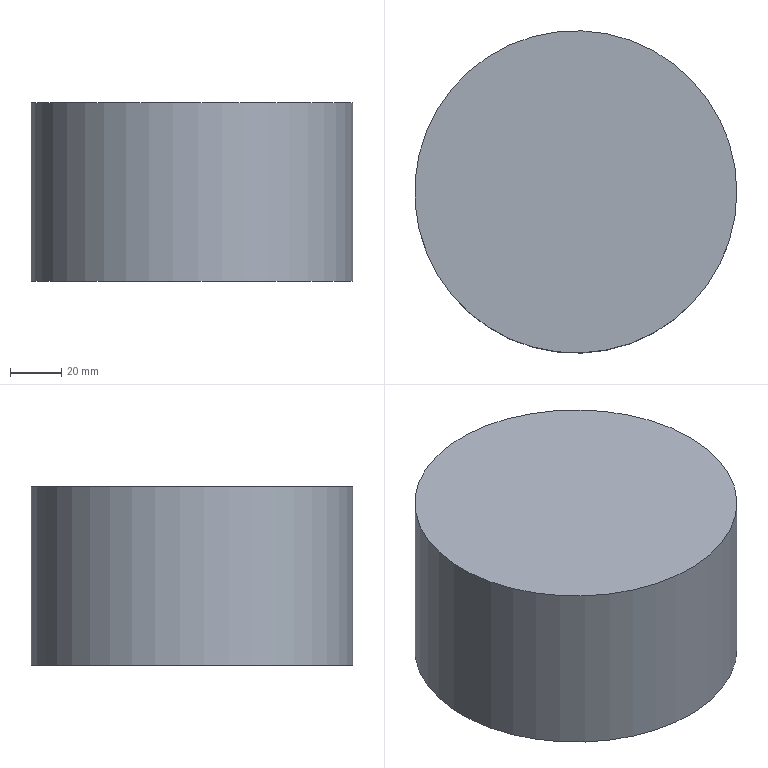Part | NX | features solid 2 | 1 solid | 5 faces | box 126 x 126 x 70 mm | volume 789734 mm3 | plane 3 | cylinder 2 | commonest cylinder face diameters 46 x1 126 x1
STEP:
#1=CARTESIAN_POINT('',(463.,230.,60.));
#2=VERTEX_POINT('',#1);
#3=CARTESIAN_POINT('',(440.,230.,60.));
#4=DIRECTION('',(0.,0.,1.));
#5=DIRECTION('',(1.,0.,0.));
#6=AXIS2_PLACEMENT_3D('',#3,#4,#5);
#7=CIRCLE('',#6,23.);
#8=EDGE_CURVE('',#2,#2,#7,.T.);
#9=ORIENTED_EDGE('',*,*,#8,.F.);
#10=EDGE_LOOP('',(#9));
#11=FACE_BOUND('',#10,.T.);
#12=CARTESIAN_POINT('',(463.,230.,110.));
#13=VERTEX_POINT('',#12);
#14=CARTESIAN_POINT('',(440.,230.,110.));
#15=DIRECTION('',(0.,0.,1.));
#16=DIRECTION('',(1.,0.,0.));
#17=AXIS2_PLACEMENT_3D('',#14,#15,#16);
#18=CIRCLE('',#17,23.);
#19=EDGE_CURVE('',#13,#13,#18,.T.);
#20=ORIENTED_EDGE('',*,*,#19,.T.);
#21=EDGE_LOOP('',(#20));
#22=FACE_BOUND('',#21,.T.);
#23=CARTESIAN_POINT('',(440.,230.,60.));
#24=DIRECTION('',(0.,0.,1.));
#25=DIRECTION('',(-1.,0.,0.));
#26=AXIS2_PLACEMENT_3D('',#23,#24,#25);
#27=CYLINDRICAL_SURFACE('',#26,23.);
#28=ADVANCED_FACE('',(#11,#22),#27,.F.);
#29=CARTESIAN_POINT('',(503.,230.,60.));
#30=VERTEX_POINT('',#29);
#31=CARTESIAN_POINT('',(440.,230.,60.));
#32=DIRECTION('',(0.,0.,1.));
#33=DIRECTION('',(1.,0.,0.));
#34=AXIS2_PLACEMENT_3D('',#31,#32,#33);
#35=CIRCLE('',#34,63.);
#36=EDGE_CURVE('',#30,#30,#35,.T.);
#37=ORIENTED_EDGE('',*,*,#36,.T.);
#38=EDGE_LOOP('',(#37));
#39=FACE_BOUND('',#38,.T.);
#40=CARTESIAN_POINT('',(503.,230.,130.));
#41=VERTEX_POINT('',#40);
#42=CARTESIAN_POINT('',(440.,230.,130.));
#43=DIRECTION('',(0.,0.,1.));
#44=DIRECTION('',(1.,0.,0.));
#45=AXIS2_PLACEMENT_3D('',#42,#43,#44);
#46=CIRCLE('',#45,63.);
#47=EDGE_CURVE('',#41,#41,#46,.T.);
#48=ORIENTED_EDGE('',*,*,#47,.F.);
#49=EDGE_LOOP('',(#48));
#50=FACE_BOUND('',#49,.T.);
#51=CARTESIAN_POINT('',(440.,230.,60.));
#52=DIRECTION('',(0.,0.,1.));
#53=DIRECTION('',(-1.,0.,0.));
#54=AXIS2_PLACEMENT_3D('',#51,#52,#53);
#55=CYLINDRICAL_SURFACE('',#54,63.);
#56=ADVANCED_FACE('',(#39,#50),#55,.T.);
#57=ORIENTED_EDGE('',*,*,#8,.T.);
#58=EDGE_LOOP('',(#57));
#59=FACE_BOUND('',#58,.T.);
#60=ORIENTED_EDGE('',*,*,#36,.F.);
#61=EDGE_LOOP('',(#60));
#62=FACE_BOUND('',#61,.T.);
#63=CARTESIAN_POINT('',(440.,230.,60.));
#64=DIRECTION('',(0.,0.,-1.));
#65=DIRECTION('',(1.,0.,0.));
#66=AXIS2_PLACEMENT_3D('',#63,#64,#65);
#67=PLANE('',#66);
#68=ADVANCED_FACE('',(#59,#62),#67,.T.);
#69=ORIENTED_EDGE('',*,*,#47,.T.);
#70=EDGE_LOOP('',(#69));
#71=FACE_BOUND('',#70,.T.);
#72=CARTESIAN_POINT('',(440.,230.,130.));
#73=DIRECTION('',(0.,0.,-1.));
#74=DIRECTION('',(1.,0.,0.));
#75=AXIS2_PLACEMENT_3D('',#72,#73,#74);
#76=PLANE('',#75);
#77=ADVANCED_FACE('',(#71),#76,.F.);
#78=ORIENTED_EDGE('',*,*,#19,.F.);
#79=EDGE_LOOP('',(#78));
#80=FACE_BOUND('',#79,.T.);
#81=CARTESIAN_POINT('',(440.,230.,110.));
#82=DIRECTION('',(0.,0.,-1.));
#83=DIRECTION('',(1.,0.,0.));
#84=AXIS2_PLACEMENT_3D('',#81,#82,#83);
#85=PLANE('',#84);
#86=ADVANCED_FACE('',(#80),#85,.T.);
#87=CLOSED_SHELL('',(#28,#56,#68,#77,#86));
#88=MANIFOLD_SOLID_BREP('',#87);
#89=(LENGTH_UNIT()NAMED_UNIT(*)SI_UNIT(.MILLI.,.METRE.));
#90=UNCERTAINTY_MEASURE_WITH_UNIT(LENGTH_MEASURE(0.00001),#89,'','');
#91=(NAMED_UNIT(*)PLANE_ANGLE_UNIT()SI_UNIT($,.RADIAN.));
#92=(NAMED_UNIT(*)SI_UNIT($,.STERADIAN.)SOLID_ANGLE_UNIT());
#93=(GEOMETRIC_REPRESENTATION_CONTEXT(3)GLOBAL_UNCERTAINTY_ASSIGNED_CONTEXT((#90))GLOBAL_UNIT_ASSIGNED_CONTEXT((#89,#91,#92))REPRESENTATION_CONTEXT('',''));
#94=ADVANCED_BREP_SHAPE_REPRESENTATION('',(#88),#93);